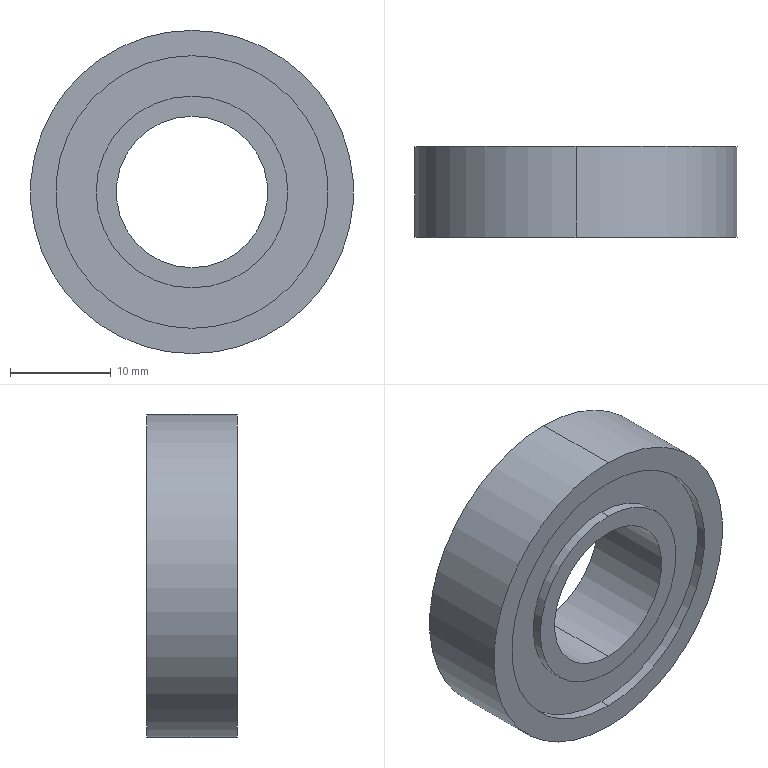Part | SolidWorks | features Revolution 1 | 1 solid | 18 faces | box 32 x 9 x 32 mm | volume 5125 mm3 | cylinder 12 | plane 6 | commonest cylinder face diameters 19 x4 27 x4 15 x2 32 x2
STEP:
#1=CARTESIAN_POINT('',(0.,-9.,-7.5));
#2=VERTEX_POINT('',#1);
#3=CARTESIAN_POINT('',(0.,-9.,7.5));
#4=VERTEX_POINT('',#3);
#5=CARTESIAN_POINT('',(0.,-9.,0.));
#6=DIRECTION('',(0.,1.,0.));
#7=DIRECTION('',(0.,0.,1.));
#8=AXIS2_PLACEMENT_3D('',#5,#6,#7);
#9=CIRCLE('',#8,7.5);
#10=EDGE_CURVE('',#2,#4,#9,.T.);
#11=ORIENTED_EDGE('',*,*,#10,.F.);
#12=CARTESIAN_POINT('',(0.,0.,-7.5));
#13=VERTEX_POINT('',#12);
#14=CARTESIAN_POINT('',(0.,13.438,-7.5));
#15=DIRECTION('',(0.,1.,0.));
#16=VECTOR('',#15,1000.);
#17=LINE('',#14,#16);
#18=EDGE_CURVE('',#2,#13,#17,.T.);
#19=ORIENTED_EDGE('',*,*,#18,.T.);
#20=CARTESIAN_POINT('',(0.,0.,7.5));
#21=VERTEX_POINT('',#20);
#22=CARTESIAN_POINT('',(0.,0.,0.));
#23=DIRECTION('',(0.,1.,0.));
#24=DIRECTION('',(0.,0.,1.));
#25=AXIS2_PLACEMENT_3D('',#22,#23,#24);
#26=CIRCLE('',#25,7.5);
#27=EDGE_CURVE('',#13,#21,#26,.T.);
#28=ORIENTED_EDGE('',*,*,#27,.T.);
#29=CARTESIAN_POINT('',(0.,13.438,7.5));
#30=DIRECTION('',(0.,1.,0.));
#31=VECTOR('',#30,1000.);
#32=LINE('',#29,#31);
#33=EDGE_CURVE('',#4,#21,#32,.T.);
#34=ORIENTED_EDGE('',*,*,#33,.F.);
#35=EDGE_LOOP('',(#11,#19,#28,#34));
#36=FACE_OUTER_BOUND('',#35,.T.);
#37=CARTESIAN_POINT('',(0.,13.438,0.));
#38=DIRECTION('',(0.,1.,0.));
#39=DIRECTION('',(0.,0.,1.));
#40=AXIS2_PLACEMENT_3D('',#37,#38,#39);
#41=CYLINDRICAL_SURFACE('',#40,7.5);
#42=ADVANCED_FACE('',(#36),#41,.F.);
#43=CARTESIAN_POINT('',(0.,-9.,9.5));
#44=VERTEX_POINT('',#43);
#45=CARTESIAN_POINT('',(0.,-9.,-9.5));
#46=VERTEX_POINT('',#45);
#47=CARTESIAN_POINT('',(0.,-9.,0.));
#48=DIRECTION('',(0.,1.,0.));
#49=DIRECTION('',(0.,0.,1.));
#50=AXIS2_PLACEMENT_3D('',#47,#48,#49);
#51=CIRCLE('',#50,9.5);
#52=EDGE_CURVE('',#44,#46,#51,.T.);
#53=ORIENTED_EDGE('',*,*,#52,.T.);
#54=CARTESIAN_POINT('',(0.,-8.,-9.5));
#55=VERTEX_POINT('',#54);
#56=CARTESIAN_POINT('',(0.,13.438,-9.5));
#57=DIRECTION('',(0.,1.,0.));
#58=VECTOR('',#57,1000.);
#59=LINE('',#56,#58);
#60=EDGE_CURVE('',#46,#55,#59,.T.);
#61=ORIENTED_EDGE('',*,*,#60,.T.);
#62=CARTESIAN_POINT('',(0.,-8.,9.5));
#63=VERTEX_POINT('',#62);
#64=CARTESIAN_POINT('',(0.,-8.,0.));
#65=DIRECTION('',(0.,1.,0.));
#66=DIRECTION('',(0.,0.,1.));
#67=AXIS2_PLACEMENT_3D('',#64,#65,#66);
#68=CIRCLE('',#67,9.5);
#69=EDGE_CURVE('',#63,#55,#68,.T.);
#70=ORIENTED_EDGE('',*,*,#69,.F.);
#71=CARTESIAN_POINT('',(0.,13.438,9.5));
#72=DIRECTION('',(0.,1.,0.));
#73=VECTOR('',#72,1000.);
#74=LINE('',#71,#73);
#75=EDGE_CURVE('',#44,#63,#74,.T.);
#76=ORIENTED_EDGE('',*,*,#75,.F.);
#77=EDGE_LOOP('',(#53,#61,#70,#76));
#78=FACE_OUTER_BOUND('',#77,.T.);
#79=CARTESIAN_POINT('',(0.,13.438,0.));
#80=DIRECTION('',(0.,1.,0.));
#81=DIRECTION('',(0.,0.,1.));
#82=AXIS2_PLACEMENT_3D('',#79,#80,#81);
#83=CYLINDRICAL_SURFACE('',#82,9.5);
#84=ADVANCED_FACE('',(#78),#83,.T.);
#85=CARTESIAN_POINT('',(0.,-9.,-13.5));
#86=VERTEX_POINT('',#85);
#87=CARTESIAN_POINT('',(0.,-9.,13.5));
#88=VERTEX_POINT('',#87);
#89=CARTESIAN_POINT('',(0.,-9.,0.));
#90=DIRECTION('',(0.,1.,0.));
#91=DIRECTION('',(0.,0.,1.));
#92=AXIS2_PLACEMENT_3D('',#89,#90,#91);
#93=CIRCLE('',#92,13.5);
#94=EDGE_CURVE('',#86,#88,#93,.T.);
#95=ORIENTED_EDGE('',*,*,#94,.F.);
#96=CARTESIAN_POINT('',(0.,-8.,-13.5));
#97=VERTEX_POINT('',#96);
#98=CARTESIAN_POINT('',(0.,13.438,-13.5));
#99=DIRECTION('',(0.,1.,0.));
#100=VECTOR('',#99,1000.);
#101=LINE('',#98,#100);
#102=EDGE_CURVE('',#86,#97,#101,.T.);
#103=ORIENTED_EDGE('',*,*,#102,.T.);
#104=CARTESIAN_POINT('',(0.,-8.,13.5));
#105=VERTEX_POINT('',#104);
#106=CARTESIAN_POINT('',(0.,-8.,0.));
#107=DIRECTION('',(0.,1.,0.));
#108=DIRECTION('',(0.,0.,1.));
#109=AXIS2_PLACEMENT_3D('',#106,#107,#108);
#110=CIRCLE('',#109,13.5);
#111=EDGE_CURVE('',#97,#105,#110,.T.);
#112=ORIENTED_EDGE('',*,*,#111,.T.);
#113=CARTESIAN_POINT('',(0.,13.438,13.5));
#114=DIRECTION('',(0.,1.,0.));
#115=VECTOR('',#114,1000.);
#116=LINE('',#113,#115);
#117=EDGE_CURVE('',#88,#105,#116,.T.);
#118=ORIENTED_EDGE('',*,*,#117,.F.);
#119=EDGE_LOOP('',(#95,#103,#112,#118));
#120=FACE_OUTER_BOUND('',#119,.T.);
#121=CARTESIAN_POINT('',(0.,13.438,0.));
#122=DIRECTION('',(0.,1.,0.));
#123=DIRECTION('',(0.,0.,1.));
#124=AXIS2_PLACEMENT_3D('',#121,#122,#123);
#125=CYLINDRICAL_SURFACE('',#124,13.5);
#126=ADVANCED_FACE('',(#120),#125,.F.);
#127=CARTESIAN_POINT('',(0.,-9.,16.));
#128=VERTEX_POINT('',#127);
#129=CARTESIAN_POINT('',(0.,-9.,-16.));
#130=VERTEX_POINT('',#129);
#131=CARTESIAN_POINT('',(0.,-9.,0.));
#132=DIRECTION('',(0.,1.,0.));
#133=DIRECTION('',(0.,0.,1.));
#134=AXIS2_PLACEMENT_3D('',#131,#132,#133);
#135=CIRCLE('',#134,16.);
#136=EDGE_CURVE('',#128,#130,#135,.T.);
#137=ORIENTED_EDGE('',*,*,#136,.T.);
#138=CARTESIAN_POINT('',(0.,0.,-16.));
#139=VERTEX_POINT('',#138);
#140=CARTESIAN_POINT('',(0.,13.438,-16.));
#141=DIRECTION('',(0.,1.,0.));
#142=VECTOR('',#141,1000.);
#143=LINE('',#140,#142);
#144=EDGE_CURVE('',#130,#139,#143,.T.);
#145=ORIENTED_EDGE('',*,*,#144,.T.);
#146=CARTESIAN_POINT('',(0.,0.,16.));
#147=VERTEX_POINT('',#146);
#148=CARTESIAN_POINT('',(0.,0.,0.));
#149=DIRECTION('',(0.,1.,0.));
#150=DIRECTION('',(0.,0.,1.));
#151=AXIS2_PLACEMENT_3D('',#148,#149,#150);
#152=CIRCLE('',#151,16.);
#153=EDGE_CURVE('',#147,#139,#152,.T.);
#154=ORIENTED_EDGE('',*,*,#153,.F.);
#155=CARTESIAN_POINT('',(0.,13.438,16.));
#156=DIRECTION('',(0.,1.,0.));
#157=VECTOR('',#156,1000.);
#158=LINE('',#155,#157);
#159=EDGE_CURVE('',#128,#147,#158,.T.);
#160=ORIENTED_EDGE('',*,*,#159,.F.);
#161=EDGE_LOOP('',(#137,#145,#154,#160));
#162=FACE_OUTER_BOUND('',#161,.T.);
#163=CARTESIAN_POINT('',(0.,13.438,0.));
#164=DIRECTION('',(0.,1.,0.));
#165=DIRECTION('',(0.,0.,1.));
#166=AXIS2_PLACEMENT_3D('',#163,#164,#165);
#167=CYLINDRICAL_SURFACE('',#166,16.);
#168=ADVANCED_FACE('',(#162),#167,.T.);
#169=CARTESIAN_POINT('',(0.,-0.8072,-13.5));
#170=VERTEX_POINT('',#169);
#171=CARTESIAN_POINT('',(0.,-0.8072,13.5));
#172=VERTEX_POINT('',#171);
#173=CARTESIAN_POINT('',(0.,-0.8072,0.));
#174=DIRECTION('',(0.,1.,0.));
#175=DIRECTION('',(0.,0.,1.));
#176=AXIS2_PLACEMENT_3D('',#173,#174,#175);
#177=CIRCLE('',#176,13.5);
#178=EDGE_CURVE('',#170,#172,#177,.T.);
#179=ORIENTED_EDGE('',*,*,#178,.F.);
#180=CARTESIAN_POINT('',(0.,0.,-13.5));
#181=VERTEX_POINT('',#180);
#182=CARTESIAN_POINT('',(0.,13.438,-13.5));
#183=DIRECTION('',(0.,1.,0.));
#184=VECTOR('',#183,1000.);
#185=LINE('',#182,#184);
#186=EDGE_CURVE('',#170,#181,#185,.T.);
#187=ORIENTED_EDGE('',*,*,#186,.T.);
#188=CARTESIAN_POINT('',(0.,0.,13.5));
#189=VERTEX_POINT('',#188);
#190=CARTESIAN_POINT('',(0.,0.,0.));
#191=DIRECTION('',(0.,1.,0.));
#192=DIRECTION('',(0.,0.,1.));
#193=AXIS2_PLACEMENT_3D('',#190,#191,#192);
#194=CIRCLE('',#193,13.5);
#195=EDGE_CURVE('',#181,#189,#194,.T.);
#196=ORIENTED_EDGE('',*,*,#195,.T.);
#197=CARTESIAN_POINT('',(0.,13.438,13.5));
#198=DIRECTION('',(0.,1.,0.));
#199=VECTOR('',#198,1000.);
#200=LINE('',#197,#199);
#201=EDGE_CURVE('',#172,#189,#200,.T.);
#202=ORIENTED_EDGE('',*,*,#201,.F.);
#203=EDGE_LOOP('',(#179,#187,#196,#202));
#204=FACE_OUTER_BOUND('',#203,.T.);
#205=CARTESIAN_POINT('',(0.,13.438,0.));
#206=DIRECTION('',(0.,1.,0.));
#207=DIRECTION('',(0.,0.,1.));
#208=AXIS2_PLACEMENT_3D('',#205,#206,#207);
#209=CYLINDRICAL_SURFACE('',#208,13.5);
#210=ADVANCED_FACE('',(#204),#209,.F.);
#211=CARTESIAN_POINT('',(0.,-0.8072,9.5));
#212=VERTEX_POINT('',#211);
#213=CARTESIAN_POINT('',(0.,-0.8072,-9.5));
#214=VERTEX_POINT('',#213);
#215=CARTESIAN_POINT('',(0.,-0.8072,0.));
#216=DIRECTION('',(0.,1.,0.));
#217=DIRECTION('',(0.,0.,1.));
#218=AXIS2_PLACEMENT_3D('',#215,#216,#217);
#219=CIRCLE('',#218,9.5);
#220=EDGE_CURVE('',#212,#214,#219,.T.);
#221=ORIENTED_EDGE('',*,*,#220,.T.);
#222=CARTESIAN_POINT('',(0.,0.,-9.5));
#223=VERTEX_POINT('',#222);
#224=CARTESIAN_POINT('',(0.,13.438,-9.5));
#225=DIRECTION('',(0.,1.,0.));
#226=VECTOR('',#225,1000.);
#227=LINE('',#224,#226);
#228=EDGE_CURVE('',#214,#223,#227,.T.);
#229=ORIENTED_EDGE('',*,*,#228,.T.);
#230=CARTESIAN_POINT('',(0.,0.,9.5));
#231=VERTEX_POINT('',#230);
#232=CARTESIAN_POINT('',(0.,0.,0.));
#233=DIRECTION('',(0.,1.,0.));
#234=DIRECTION('',(0.,0.,1.));
#235=AXIS2_PLACEMENT_3D('',#232,#233,#234);
#236=CIRCLE('',#235,9.5);
#237=EDGE_CURVE('',#231,#223,#236,.T.);
#238=ORIENTED_EDGE('',*,*,#237,.F.);
#239=CARTESIAN_POINT('',(0.,13.438,9.5));
#240=DIRECTION('',(0.,1.,0.));
#241=VECTOR('',#240,1000.);
#242=LINE('',#239,#241);
#243=EDGE_CURVE('',#212,#231,#242,.T.);
#244=ORIENTED_EDGE('',*,*,#243,.F.);
#245=EDGE_LOOP('',(#221,#229,#238,#244));
#246=FACE_OUTER_BOUND('',#245,.T.);
#247=CARTESIAN_POINT('',(0.,13.438,0.));
#248=DIRECTION('',(0.,1.,0.));
#249=DIRECTION('',(0.,0.,1.));
#250=AXIS2_PLACEMENT_3D('',#247,#248,#249);
#251=CYLINDRICAL_SURFACE('',#250,9.5);
#252=ADVANCED_FACE('',(#246),#251,.T.);
#253=CARTESIAN_POINT('',(0.,0.,0.));
#254=DIRECTION('',(0.,1.,0.));
#255=DIRECTION('',(0.,0.,1.));
#256=AXIS2_PLACEMENT_3D('',#253,#254,#255);
#257=CIRCLE('',#256,7.5);
#258=EDGE_CURVE('',#21,#13,#257,.T.);
#259=ORIENTED_EDGE('',*,*,#258,.F.);
#260=ORIENTED_EDGE('',*,*,#27,.F.);
#261=EDGE_LOOP('',(#259,#260));
#262=FACE_BOUND('',#261,.T.);
#263=ORIENTED_EDGE('',*,*,#237,.T.);
#264=CARTESIAN_POINT('',(0.,0.,0.));
#265=DIRECTION('',(0.,1.,0.));
#266=DIRECTION('',(0.,0.,1.));
#267=AXIS2_PLACEMENT_3D('',#264,#265,#266);
#268=CIRCLE('',#267,9.5);
#269=EDGE_CURVE('',#223,#231,#268,.T.);
#270=ORIENTED_EDGE('',*,*,#269,.T.);
#271=EDGE_LOOP('',(#263,#270));
#272=FACE_OUTER_BOUND('',#271,.T.);
#273=CARTESIAN_POINT('',(7.5,0.,0.));
#274=DIRECTION('',(0.,-1.,0.));
#275=DIRECTION('',(0.,0.,-1.));
#276=AXIS2_PLACEMENT_3D('',#273,#274,#275);
#277=PLANE('',#276);
#278=ADVANCED_FACE('',(#262,#272),#277,.F.);
#279=ORIENTED_EDGE('',*,*,#228,.F.);
#280=CARTESIAN_POINT('',(0.,-0.8072,0.));
#281=DIRECTION('',(0.,1.,0.));
#282=DIRECTION('',(0.,0.,1.));
#283=AXIS2_PLACEMENT_3D('',#280,#281,#282);
#284=CIRCLE('',#283,9.5);
#285=EDGE_CURVE('',#214,#212,#284,.T.);
#286=ORIENTED_EDGE('',*,*,#285,.T.);
#287=ORIENTED_EDGE('',*,*,#243,.T.);
#288=ORIENTED_EDGE('',*,*,#269,.F.);
#289=EDGE_LOOP('',(#279,#286,#287,#288));
#290=FACE_OUTER_BOUND('',#289,.T.);
#291=CARTESIAN_POINT('',(0.,13.438,0.));
#292=DIRECTION('',(0.,1.,0.));
#293=DIRECTION('',(0.,0.,1.));
#294=AXIS2_PLACEMENT_3D('',#291,#292,#293);
#295=CYLINDRICAL_SURFACE('',#294,9.5);
#296=ADVANCED_FACE('',(#290),#295,.T.);
#297=ORIENTED_EDGE('',*,*,#220,.F.);
#298=ORIENTED_EDGE('',*,*,#285,.F.);
#299=EDGE_LOOP('',(#297,#298));
#300=FACE_BOUND('',#299,.T.);
#301=CARTESIAN_POINT('',(0.,-0.8072,0.));
#302=DIRECTION('',(0.,1.,0.));
#303=DIRECTION('',(0.,0.,1.));
#304=AXIS2_PLACEMENT_3D('',#301,#302,#303);
#305=CIRCLE('',#304,13.5);
#306=EDGE_CURVE('',#172,#170,#305,.T.);
#307=ORIENTED_EDGE('',*,*,#306,.T.);
#308=ORIENTED_EDGE('',*,*,#178,.T.);
#309=EDGE_LOOP('',(#307,#308));
#310=FACE_OUTER_BOUND('',#309,.T.);
#311=CARTESIAN_POINT('',(9.5,-0.8072,0.));
#312=DIRECTION('',(0.,-1.,0.));
#313=DIRECTION('',(0.,0.,-1.));
#314=AXIS2_PLACEMENT_3D('',#311,#312,#313);
#315=PLANE('',#314);
#316=ADVANCED_FACE('',(#300,#310),#315,.F.);
#317=ORIENTED_EDGE('',*,*,#186,.F.);
#318=ORIENTED_EDGE('',*,*,#306,.F.);
#319=ORIENTED_EDGE('',*,*,#201,.T.);
#320=CARTESIAN_POINT('',(0.,0.,0.));
#321=DIRECTION('',(0.,1.,0.));
#322=DIRECTION('',(0.,0.,1.));
#323=AXIS2_PLACEMENT_3D('',#320,#321,#322);
#324=CIRCLE('',#323,13.5);
#325=EDGE_CURVE('',#189,#181,#324,.T.);
#326=ORIENTED_EDGE('',*,*,#325,.T.);
#327=EDGE_LOOP('',(#317,#318,#319,#326));
#328=FACE_OUTER_BOUND('',#327,.T.);
#329=CARTESIAN_POINT('',(0.,13.438,0.));
#330=DIRECTION('',(0.,1.,0.));
#331=DIRECTION('',(0.,0.,1.));
#332=AXIS2_PLACEMENT_3D('',#329,#330,#331);
#333=CYLINDRICAL_SURFACE('',#332,13.5);
#334=ADVANCED_FACE('',(#328),#333,.F.);
#335=ORIENTED_EDGE('',*,*,#325,.F.);
#336=ORIENTED_EDGE('',*,*,#195,.F.);
#337=EDGE_LOOP('',(#335,#336));
#338=FACE_BOUND('',#337,.T.);
#339=ORIENTED_EDGE('',*,*,#153,.T.);
#340=CARTESIAN_POINT('',(0.,0.,0.));
#341=DIRECTION('',(0.,1.,0.));
#342=DIRECTION('',(0.,0.,1.));
#343=AXIS2_PLACEMENT_3D('',#340,#341,#342);
#344=CIRCLE('',#343,16.);
#345=EDGE_CURVE('',#139,#147,#344,.T.);
#346=ORIENTED_EDGE('',*,*,#345,.T.);
#347=EDGE_LOOP('',(#339,#346));
#348=FACE_OUTER_BOUND('',#347,.T.);
#349=CARTESIAN_POINT('',(13.5,0.,0.));
#350=DIRECTION('',(0.,-1.,0.));
#351=DIRECTION('',(0.,0.,-1.));
#352=AXIS2_PLACEMENT_3D('',#349,#350,#351);
#353=PLANE('',#352);
#354=ADVANCED_FACE('',(#338,#348),#353,.F.);
#355=ORIENTED_EDGE('',*,*,#144,.F.);
#356=CARTESIAN_POINT('',(0.,-9.,0.));
#357=DIRECTION('',(0.,1.,0.));
#358=DIRECTION('',(0.,0.,1.));
#359=AXIS2_PLACEMENT_3D('',#356,#357,#358);
#360=CIRCLE('',#359,16.);
#361=EDGE_CURVE('',#130,#128,#360,.T.);
#362=ORIENTED_EDGE('',*,*,#361,.T.);
#363=ORIENTED_EDGE('',*,*,#159,.T.);
#364=ORIENTED_EDGE('',*,*,#345,.F.);
#365=EDGE_LOOP('',(#355,#362,#363,#364));
#366=FACE_OUTER_BOUND('',#365,.T.);
#367=CARTESIAN_POINT('',(0.,13.438,0.));
#368=DIRECTION('',(0.,1.,0.));
#369=DIRECTION('',(0.,0.,1.));
#370=AXIS2_PLACEMENT_3D('',#367,#368,#369);
#371=CYLINDRICAL_SURFACE('',#370,16.);
#372=ADVANCED_FACE('',(#366),#371,.T.);
#373=ORIENTED_EDGE('',*,*,#136,.F.);
#374=ORIENTED_EDGE('',*,*,#361,.F.);
#375=EDGE_LOOP('',(#373,#374));
#376=FACE_OUTER_BOUND('',#375,.T.);
#377=CARTESIAN_POINT('',(0.,-9.,0.));
#378=DIRECTION('',(0.,1.,0.));
#379=DIRECTION('',(0.,0.,1.));
#380=AXIS2_PLACEMENT_3D('',#377,#378,#379);
#381=CIRCLE('',#380,13.5);
#382=EDGE_CURVE('',#88,#86,#381,.T.);
#383=ORIENTED_EDGE('',*,*,#382,.T.);
#384=ORIENTED_EDGE('',*,*,#94,.T.);
#385=EDGE_LOOP('',(#383,#384));
#386=FACE_BOUND('',#385,.T.);
#387=CARTESIAN_POINT('',(13.5,-9.,0.));
#388=DIRECTION('',(0.,1.,0.));
#389=DIRECTION('',(0.,0.,1.));
#390=AXIS2_PLACEMENT_3D('',#387,#388,#389);
#391=PLANE('',#390);
#392=ADVANCED_FACE('',(#376,#386),#391,.F.);
#393=ORIENTED_EDGE('',*,*,#102,.F.);
#394=ORIENTED_EDGE('',*,*,#382,.F.);
#395=ORIENTED_EDGE('',*,*,#117,.T.);
#396=CARTESIAN_POINT('',(0.,-8.,0.));
#397=DIRECTION('',(0.,1.,0.));
#398=DIRECTION('',(0.,0.,1.));
#399=AXIS2_PLACEMENT_3D('',#396,#397,#398);
#400=CIRCLE('',#399,13.5);
#401=EDGE_CURVE('',#105,#97,#400,.T.);
#402=ORIENTED_EDGE('',*,*,#401,.T.);
#403=EDGE_LOOP('',(#393,#394,#395,#402));
#404=FACE_OUTER_BOUND('',#403,.T.);
#405=CARTESIAN_POINT('',(0.,13.438,0.));
#406=DIRECTION('',(0.,1.,0.));
#407=DIRECTION('',(0.,0.,1.));
#408=AXIS2_PLACEMENT_3D('',#405,#406,#407);
#409=CYLINDRICAL_SURFACE('',#408,13.5);
#410=ADVANCED_FACE('',(#404),#409,.F.);
#411=ORIENTED_EDGE('',*,*,#401,.F.);
#412=ORIENTED_EDGE('',*,*,#111,.F.);
#413=EDGE_LOOP('',(#411,#412));
#414=FACE_OUTER_BOUND('',#413,.T.);
#415=ORIENTED_EDGE('',*,*,#69,.T.);
#416=CARTESIAN_POINT('',(0.,-8.,0.));
#417=DIRECTION('',(0.,1.,0.));
#418=DIRECTION('',(0.,0.,1.));
#419=AXIS2_PLACEMENT_3D('',#416,#417,#418);
#420=CIRCLE('',#419,9.5);
#421=EDGE_CURVE('',#55,#63,#420,.T.);
#422=ORIENTED_EDGE('',*,*,#421,.T.);
#423=EDGE_LOOP('',(#415,#422));
#424=FACE_BOUND('',#423,.T.);
#425=CARTESIAN_POINT('',(9.5,-8.,0.));
#426=DIRECTION('',(0.,1.,0.));
#427=DIRECTION('',(0.,0.,1.));
#428=AXIS2_PLACEMENT_3D('',#425,#426,#427);
#429=PLANE('',#428);
#430=ADVANCED_FACE('',(#414,#424),#429,.F.);
#431=ORIENTED_EDGE('',*,*,#60,.F.);
#432=CARTESIAN_POINT('',(0.,-9.,0.));
#433=DIRECTION('',(0.,1.,0.));
#434=DIRECTION('',(0.,0.,1.));
#435=AXIS2_PLACEMENT_3D('',#432,#433,#434);
#436=CIRCLE('',#435,9.5);
#437=EDGE_CURVE('',#46,#44,#436,.T.);
#438=ORIENTED_EDGE('',*,*,#437,.T.);
#439=ORIENTED_EDGE('',*,*,#75,.T.);
#440=ORIENTED_EDGE('',*,*,#421,.F.);
#441=EDGE_LOOP('',(#431,#438,#439,#440));
#442=FACE_OUTER_BOUND('',#441,.T.);
#443=CARTESIAN_POINT('',(0.,13.438,0.));
#444=DIRECTION('',(0.,1.,0.));
#445=DIRECTION('',(0.,0.,1.));
#446=AXIS2_PLACEMENT_3D('',#443,#444,#445);
#447=CYLINDRICAL_SURFACE('',#446,9.5);
#448=ADVANCED_FACE('',(#442),#447,.T.);
#449=ORIENTED_EDGE('',*,*,#52,.F.);
#450=ORIENTED_EDGE('',*,*,#437,.F.);
#451=EDGE_LOOP('',(#449,#450));
#452=FACE_OUTER_BOUND('',#451,.T.);
#453=CARTESIAN_POINT('',(0.,-9.,0.));
#454=DIRECTION('',(0.,1.,0.));
#455=DIRECTION('',(0.,0.,1.));
#456=AXIS2_PLACEMENT_3D('',#453,#454,#455);
#457=CIRCLE('',#456,7.5);
#458=EDGE_CURVE('',#4,#2,#457,.T.);
#459=ORIENTED_EDGE('',*,*,#458,.T.);
#460=ORIENTED_EDGE('',*,*,#10,.T.);
#461=EDGE_LOOP('',(#459,#460));
#462=FACE_BOUND('',#461,.T.);
#463=CARTESIAN_POINT('',(7.5,-9.,0.));
#464=DIRECTION('',(0.,1.,0.));
#465=DIRECTION('',(0.,0.,1.));
#466=AXIS2_PLACEMENT_3D('',#463,#464,#465);
#467=PLANE('',#466);
#468=ADVANCED_FACE('',(#452,#462),#467,.F.);
#469=ORIENTED_EDGE('',*,*,#18,.F.);
#470=ORIENTED_EDGE('',*,*,#458,.F.);
#471=ORIENTED_EDGE('',*,*,#33,.T.);
#472=ORIENTED_EDGE('',*,*,#258,.T.);
#473=EDGE_LOOP('',(#469,#470,#471,#472));
#474=FACE_OUTER_BOUND('',#473,.T.);
#475=CARTESIAN_POINT('',(0.,13.438,0.));
#476=DIRECTION('',(0.,1.,0.));
#477=DIRECTION('',(0.,0.,1.));
#478=AXIS2_PLACEMENT_3D('',#475,#476,#477);
#479=CYLINDRICAL_SURFACE('',#478,7.5);
#480=ADVANCED_FACE('',(#474),#479,.F.);
#481=CLOSED_SHELL('',(#42,#84,#126,#168,#210,#252,#278,#296,#316,#334,#354,#372,#392,#410,#430,#448,#468,#480));
#482=MANIFOLD_SOLID_BREP('',#481);
#483=CARTESIAN_POINT('',(0.,0.,0.));
#484=DIRECTION('',(0.,0.,1.));
#485=DIRECTION('',(1.,0.,0.));
#486=AXIS2_PLACEMENT_3D('',#483,#484,#485);
#487=(LENGTH_UNIT()NAMED_UNIT(*)SI_UNIT(.MILLI.,.METRE.));
#488=UNCERTAINTY_MEASURE_WITH_UNIT(LENGTH_MEASURE(0.00001),#487,'','');
#489=(NAMED_UNIT(*)PLANE_ANGLE_UNIT()SI_UNIT($,.RADIAN.));
#490=(NAMED_UNIT(*)SI_UNIT($,.STERADIAN.)SOLID_ANGLE_UNIT());
#491=(GEOMETRIC_REPRESENTATION_CONTEXT(3)GLOBAL_UNCERTAINTY_ASSIGNED_CONTEXT((#488))GLOBAL_UNIT_ASSIGNED_CONTEXT((#487,#489,#490))REPRESENTATION_CONTEXT('',''));
#492=ADVANCED_BREP_SHAPE_REPRESENTATION('',(#482,#486),#491);